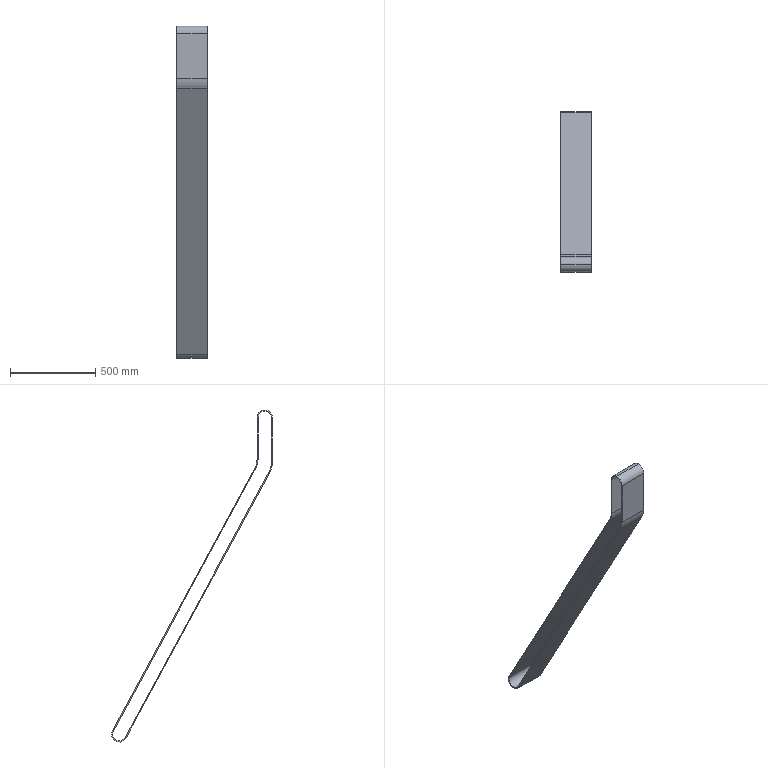Part | NX | 1 solid | 20 faces | box 180 x 945 x 1950 mm | volume 4768018 mm3 | cylinder 10 | plane 10 | commonest cylinder face diameters 78 x3 90 x3 240 x2 228 x1 252 x1
STEP:
#1=CARTESIAN_POINT('',(220.674,-610.499,2425.086));
#2=VERTEX_POINT('',#1);
#3=CARTESIAN_POINT('',(220.674,-649.499,2464.086));
#4=VERTEX_POINT('',#3);
#5=CARTESIAN_POINT('',(220.674,-649.499,2425.086));
#6=DIRECTION('',(1.,0.,0.));
#7=DIRECTION('',(0.,0.,-1.));
#8=AXIS2_PLACEMENT_3D('',#5,#6,#7);
#9=CIRCLE('',#8,39.);
#10=EDGE_CURVE('',#2,#4,#9,.T.);
#11=ORIENTED_EDGE('',*,*,#10,.T.);
#12=CARTESIAN_POINT('',(40.674,-649.499,2464.086));
#13=VERTEX_POINT('',#12);
#14=CARTESIAN_POINT('',(220.674,-649.499,2464.086));
#15=DIRECTION('',(-1.,0.,0.));
#16=VECTOR('',#15,1.);
#17=LINE('',#14,#16);
#18=EDGE_CURVE('',#4,#13,#17,.T.);
#19=ORIENTED_EDGE('',*,*,#18,.T.);
#20=CARTESIAN_POINT('',(40.674,-610.499,2425.086));
#21=VERTEX_POINT('',#20);
#22=CARTESIAN_POINT('',(40.674,-649.499,2425.086));
#23=DIRECTION('',(1.,0.,0.));
#24=DIRECTION('',(0.,0.,-1.));
#25=AXIS2_PLACEMENT_3D('',#22,#23,#24);
#26=CIRCLE('',#25,39.);
#27=EDGE_CURVE('',#21,#13,#26,.T.);
#28=ORIENTED_EDGE('',*,*,#27,.F.);
#29=CARTESIAN_POINT('',(220.674,-610.499,2425.086));
#30=DIRECTION('',(-1.,0.,0.));
#31=VECTOR('',#30,1.);
#32=LINE('',#29,#31);
#33=EDGE_CURVE('',#2,#21,#32,.T.);
#34=ORIENTED_EDGE('',*,*,#33,.F.);
#35=EDGE_LOOP('',(#11,#19,#28,#34));
#36=FACE_OUTER_BOUND('',#35,.T.);
#37=CARTESIAN_POINT('',(220.674,-649.499,2425.086));
#38=DIRECTION('',(-1.,0.,0.));
#39=DIRECTION('',(0.,0.,1.));
#40=AXIS2_PLACEMENT_3D('',#37,#38,#39);
#41=CYLINDRICAL_SURFACE('',#40,39.);
#42=ADVANCED_FACE('',(#36),#41,.F.);
#43=CARTESIAN_POINT('',(220.674,-649.499,2470.086));
#44=VERTEX_POINT('',#43);
#45=CARTESIAN_POINT('',(220.674,-694.499,2425.086));
#46=VERTEX_POINT('',#45);
#47=CARTESIAN_POINT('',(220.674,-649.499,2425.086));
#48=DIRECTION('',(1.,0.,0.));
#49=DIRECTION('',(0.,0.,-1.));
#50=AXIS2_PLACEMENT_3D('',#47,#48,#49);
#51=CIRCLE('',#50,45.);
#52=EDGE_CURVE('',#44,#46,#51,.T.);
#53=ORIENTED_EDGE('',*,*,#52,.F.);
#54=CARTESIAN_POINT('',(40.674,-649.499,2470.086));
#55=VERTEX_POINT('',#54);
#56=CARTESIAN_POINT('',(220.674,-649.499,2470.086));
#57=DIRECTION('',(-1.,0.,0.));
#58=VECTOR('',#57,1.);
#59=LINE('',#56,#58);
#60=EDGE_CURVE('',#44,#55,#59,.T.);
#61=ORIENTED_EDGE('',*,*,#60,.T.);
#62=CARTESIAN_POINT('',(40.674,-694.499,2425.086));
#63=VERTEX_POINT('',#62);
#64=CARTESIAN_POINT('',(40.674,-649.499,2425.086));
#65=DIRECTION('',(1.,0.,0.));
#66=DIRECTION('',(0.,0.,-1.));
#67=AXIS2_PLACEMENT_3D('',#64,#65,#66);
#68=CIRCLE('',#67,45.);
#69=EDGE_CURVE('',#55,#63,#68,.T.);
#70=ORIENTED_EDGE('',*,*,#69,.T.);
#71=CARTESIAN_POINT('',(220.674,-694.499,2425.086));
#72=DIRECTION('',(-1.,0.,0.));
#73=VECTOR('',#72,1.);
#74=LINE('',#71,#73);
#75=EDGE_CURVE('',#46,#63,#74,.T.);
#76=ORIENTED_EDGE('',*,*,#75,.F.);
#77=EDGE_LOOP('',(#53,#61,#70,#76));
#78=FACE_OUTER_BOUND('',#77,.T.);
#79=CARTESIAN_POINT('',(220.674,-649.499,2425.086));
#80=DIRECTION('',(-1.,0.,0.));
#81=DIRECTION('',(0.,0.,1.));
#82=AXIS2_PLACEMENT_3D('',#79,#80,#81);
#83=CYLINDRICAL_SURFACE('',#82,45.);
#84=ADVANCED_FACE('',(#78),#83,.T.);
#85=CARTESIAN_POINT('',(220.674,-590.01,2127.924));
#86=VERTEX_POINT('',#85);
#87=CARTESIAN_POINT('',(220.674,-604.499,2185.086));
#88=VERTEX_POINT('',#87);
#89=CARTESIAN_POINT('',(220.674,-484.499,2185.086));
#90=DIRECTION('',(-1.,0.,0.));
#91=DIRECTION('',(0.,0.,-1.));
#92=AXIS2_PLACEMENT_3D('',#89,#90,#91);
#93=CIRCLE('',#92,120.);
#94=EDGE_CURVE('',#86,#88,#93,.T.);
#95=ORIENTED_EDGE('',*,*,#94,.T.);
#96=CARTESIAN_POINT('',(220.674,-604.499,2425.086));
#97=VERTEX_POINT('',#96);
#98=CARTESIAN_POINT('',(220.674,-604.499,2425.086));
#99=DIRECTION('',(0.,0.,1.));
#100=VECTOR('',#99,1.);
#101=LINE('',#98,#100);
#102=EDGE_CURVE('',#88,#97,#101,.T.);
#103=ORIENTED_EDGE('',*,*,#102,.T.);
#104=CARTESIAN_POINT('',(220.674,-649.499,2425.086));
#105=DIRECTION('',(1.,0.,0.));
#106=DIRECTION('',(0.,0.,-1.));
#107=AXIS2_PLACEMENT_3D('',#104,#105,#106);
#108=CIRCLE('',#107,45.);
#109=EDGE_CURVE('',#97,#44,#108,.T.);
#110=ORIENTED_EDGE('',*,*,#109,.T.);
#111=ORIENTED_EDGE('',*,*,#52,.T.);
#112=CARTESIAN_POINT('',(220.674,-694.499,2162.273));
#113=VERTEX_POINT('',#112);
#114=CARTESIAN_POINT('',(220.674,-694.499,2162.273));
#115=DIRECTION('',(0.,0.,-1.));
#116=VECTOR('',#115,1.);
#117=LINE('',#114,#116);
#118=EDGE_CURVE('',#46,#113,#117,.T.);
#119=ORIENTED_EDGE('',*,*,#118,.T.);
#120=CARTESIAN_POINT('',(220.674,-680.01,2105.111));
#121=VERTEX_POINT('',#120);
#122=CARTESIAN_POINT('',(220.674,-574.499,2162.273));
#123=DIRECTION('',(1.,0.,0.));
#124=DIRECTION('',(0.,0.,1.));
#125=AXIS2_PLACEMENT_3D('',#122,#123,#124);
#126=CIRCLE('',#125,120.);
#127=EDGE_CURVE('',#113,#121,#126,.T.);
#128=ORIENTED_EDGE('',*,*,#127,.T.);
#129=CARTESIAN_POINT('',(220.674,165.934,543.65));
#130=VERTEX_POINT('',#129);
#131=CARTESIAN_POINT('',(220.674,165.934,543.65));
#132=DIRECTION('',(0.,0.4763,-0.8793));
#133=VECTOR('',#132,1.);
#134=LINE('',#131,#133);
#135=EDGE_CURVE('',#121,#130,#134,.T.);
#136=ORIENTED_EDGE('',*,*,#135,.T.);
#137=CARTESIAN_POINT('',(220.674,245.067,586.522));
#138=VERTEX_POINT('',#137);
#139=CARTESIAN_POINT('',(220.674,205.501,565.086));
#140=DIRECTION('',(1.,0.,0.));
#141=DIRECTION('',(0.,0.,1.));
#142=AXIS2_PLACEMENT_3D('',#139,#140,#141);
#143=CIRCLE('',#142,45.);
#144=EDGE_CURVE('',#130,#138,#143,.T.);
#145=ORIENTED_EDGE('',*,*,#144,.T.);
#146=CARTESIAN_POINT('',(220.674,-590.01,2127.924));
#147=DIRECTION('',(0.,-0.4763,0.8793));
#148=VECTOR('',#147,1.);
#149=LINE('',#146,#148);
#150=EDGE_CURVE('',#138,#86,#149,.T.);
#151=ORIENTED_EDGE('',*,*,#150,.T.);
#152=EDGE_LOOP('',(#95,#103,#110,#111,#119,#128,#136,#145,#151));
#153=FACE_BOUND('',#152,.T.);
#154=CARTESIAN_POINT('',(220.674,-595.286,2125.066));
#155=VERTEX_POINT('',#154);
#156=CARTESIAN_POINT('',(220.674,-610.499,2185.086));
#157=VERTEX_POINT('',#156);
#158=CARTESIAN_POINT('',(220.674,-484.499,2185.086));
#159=DIRECTION('',(-1.,0.,0.));
#160=DIRECTION('',(0.,0.,-1.));
#161=AXIS2_PLACEMENT_3D('',#158,#159,#160);
#162=CIRCLE('',#161,126.);
#163=EDGE_CURVE('',#155,#157,#162,.T.);
#164=ORIENTED_EDGE('',*,*,#163,.F.);
#165=CARTESIAN_POINT('',(220.674,239.792,583.664));
#166=VERTEX_POINT('',#165);
#167=CARTESIAN_POINT('',(220.674,-595.286,2125.066));
#168=DIRECTION('',(0.,-0.4763,0.8793));
#169=VECTOR('',#168,1.);
#170=LINE('',#167,#169);
#171=EDGE_CURVE('',#166,#155,#170,.T.);
#172=ORIENTED_EDGE('',*,*,#171,.F.);
#173=CARTESIAN_POINT('',(220.674,171.21,546.509));
#174=VERTEX_POINT('',#173);
#175=CARTESIAN_POINT('',(220.674,205.501,565.086));
#176=DIRECTION('',(1.,0.,0.));
#177=DIRECTION('',(0.,0.,-1.));
#178=AXIS2_PLACEMENT_3D('',#175,#176,#177);
#179=CIRCLE('',#178,39.);
#180=EDGE_CURVE('',#174,#166,#179,.T.);
#181=ORIENTED_EDGE('',*,*,#180,.F.);
#182=CARTESIAN_POINT('',(220.674,-674.734,2107.969));
#183=VERTEX_POINT('',#182);
#184=CARTESIAN_POINT('',(220.674,171.21,546.509));
#185=DIRECTION('',(0.,0.4763,-0.8793));
#186=VECTOR('',#185,1.);
#187=LINE('',#184,#186);
#188=EDGE_CURVE('',#183,#174,#187,.T.);
#189=ORIENTED_EDGE('',*,*,#188,.F.);
#190=CARTESIAN_POINT('',(220.674,-688.499,2162.273));
#191=VERTEX_POINT('',#190);
#192=CARTESIAN_POINT('',(220.674,-574.499,2162.273));
#193=DIRECTION('',(1.,0.,0.));
#194=DIRECTION('',(0.,0.,-1.));
#195=AXIS2_PLACEMENT_3D('',#192,#193,#194);
#196=CIRCLE('',#195,114.);
#197=EDGE_CURVE('',#191,#183,#196,.T.);
#198=ORIENTED_EDGE('',*,*,#197,.F.);
#199=CARTESIAN_POINT('',(220.674,-688.499,2425.086));
#200=VERTEX_POINT('',#199);
#201=CARTESIAN_POINT('',(220.674,-688.499,2162.273));
#202=DIRECTION('',(0.,0.,-1.));
#203=VECTOR('',#202,1.);
#204=LINE('',#201,#203);
#205=EDGE_CURVE('',#200,#191,#204,.T.);
#206=ORIENTED_EDGE('',*,*,#205,.F.);
#207=CARTESIAN_POINT('',(220.674,-649.499,2425.086));
#208=DIRECTION('',(1.,0.,0.));
#209=DIRECTION('',(0.,0.,-1.));
#210=AXIS2_PLACEMENT_3D('',#207,#208,#209);
#211=CIRCLE('',#210,39.);
#212=EDGE_CURVE('',#4,#200,#211,.T.);
#213=ORIENTED_EDGE('',*,*,#212,.F.);
#214=ORIENTED_EDGE('',*,*,#10,.F.);
#215=CARTESIAN_POINT('',(220.674,-610.499,2425.086));
#216=DIRECTION('',(0.,0.,1.));
#217=VECTOR('',#216,1.);
#218=LINE('',#215,#217);
#219=EDGE_CURVE('',#157,#2,#218,.T.);
#220=ORIENTED_EDGE('',*,*,#219,.F.);
#221=EDGE_LOOP('',(#164,#172,#181,#189,#198,#206,#213,#214,#220));
#222=FACE_BOUND('',#221,.T.);
#223=CARTESIAN_POINT('',(220.674,-484.499,2185.086));
#224=DIRECTION('',(-1.,0.,0.));
#225=DIRECTION('',(0.,0.,1.));
#226=AXIS2_PLACEMENT_3D('',#223,#224,#225);
#227=PLANE('',#226);
#228=ADVANCED_FACE('',(#153,#222),#227,.F.);
#229=CARTESIAN_POINT('',(40.674,-590.01,2127.924));
#230=VERTEX_POINT('',#229);
#231=CARTESIAN_POINT('',(40.674,-604.499,2185.086));
#232=VERTEX_POINT('',#231);
#233=CARTESIAN_POINT('',(40.674,-484.499,2185.086));
#234=DIRECTION('',(-1.,0.,0.));
#235=DIRECTION('',(0.,0.,-1.));
#236=AXIS2_PLACEMENT_3D('',#233,#234,#235);
#237=CIRCLE('',#236,120.);
#238=EDGE_CURVE('',#230,#232,#237,.T.);
#239=ORIENTED_EDGE('',*,*,#238,.F.);
#240=CARTESIAN_POINT('',(40.674,245.067,586.522));
#241=VERTEX_POINT('',#240);
#242=CARTESIAN_POINT('',(40.674,-590.01,2127.924));
#243=DIRECTION('',(0.,-0.4763,0.8793));
#244=VECTOR('',#243,1.);
#245=LINE('',#242,#244);
#246=EDGE_CURVE('',#241,#230,#245,.T.);
#247=ORIENTED_EDGE('',*,*,#246,.F.);
#248=CARTESIAN_POINT('',(40.674,165.934,543.65));
#249=VERTEX_POINT('',#248);
#250=CARTESIAN_POINT('',(40.674,205.501,565.086));
#251=DIRECTION('',(1.,0.,0.));
#252=DIRECTION('',(0.,0.,1.));
#253=AXIS2_PLACEMENT_3D('',#250,#251,#252);
#254=CIRCLE('',#253,45.);
#255=EDGE_CURVE('',#249,#241,#254,.T.);
#256=ORIENTED_EDGE('',*,*,#255,.F.);
#257=CARTESIAN_POINT('',(40.674,-680.01,2105.111));
#258=VERTEX_POINT('',#257);
#259=CARTESIAN_POINT('',(40.674,165.934,543.65));
#260=DIRECTION('',(0.,0.4763,-0.8793));
#261=VECTOR('',#260,1.);
#262=LINE('',#259,#261);
#263=EDGE_CURVE('',#258,#249,#262,.T.);
#264=ORIENTED_EDGE('',*,*,#263,.F.);
#265=CARTESIAN_POINT('',(40.674,-694.499,2162.273));
#266=VERTEX_POINT('',#265);
#267=CARTESIAN_POINT('',(40.674,-574.499,2162.273));
#268=DIRECTION('',(1.,0.,0.));
#269=DIRECTION('',(0.,0.,1.));
#270=AXIS2_PLACEMENT_3D('',#267,#268,#269);
#271=CIRCLE('',#270,120.);
#272=EDGE_CURVE('',#266,#258,#271,.T.);
#273=ORIENTED_EDGE('',*,*,#272,.F.);
#274=CARTESIAN_POINT('',(40.674,-694.499,2162.273));
#275=DIRECTION('',(0.,0.,-1.));
#276=VECTOR('',#275,1.);
#277=LINE('',#274,#276);
#278=EDGE_CURVE('',#63,#266,#277,.T.);
#279=ORIENTED_EDGE('',*,*,#278,.F.);
#280=ORIENTED_EDGE('',*,*,#69,.F.);
#281=CARTESIAN_POINT('',(40.674,-604.499,2425.086));
#282=VERTEX_POINT('',#281);
#283=CARTESIAN_POINT('',(40.674,-649.499,2425.086));
#284=DIRECTION('',(1.,0.,0.));
#285=DIRECTION('',(0.,0.,-1.));
#286=AXIS2_PLACEMENT_3D('',#283,#284,#285);
#287=CIRCLE('',#286,45.);
#288=EDGE_CURVE('',#282,#55,#287,.T.);
#289=ORIENTED_EDGE('',*,*,#288,.F.);
#290=CARTESIAN_POINT('',(40.674,-604.499,2425.086));
#291=DIRECTION('',(0.,0.,1.));
#292=VECTOR('',#291,1.);
#293=LINE('',#290,#292);
#294=EDGE_CURVE('',#232,#282,#293,.T.);
#295=ORIENTED_EDGE('',*,*,#294,.F.);
#296=EDGE_LOOP('',(#239,#247,#256,#264,#273,#279,#280,#289,#295));
#297=FACE_BOUND('',#296,.T.);
#298=CARTESIAN_POINT('',(40.674,239.792,583.664));
#299=VERTEX_POINT('',#298);
#300=CARTESIAN_POINT('',(40.674,-595.286,2125.066));
#301=VERTEX_POINT('',#300);
#302=CARTESIAN_POINT('',(40.674,-595.286,2125.066));
#303=DIRECTION('',(0.,-0.4763,0.8793));
#304=VECTOR('',#303,1.);
#305=LINE('',#302,#304);
#306=EDGE_CURVE('',#299,#301,#305,.T.);
#307=ORIENTED_EDGE('',*,*,#306,.T.);
#308=CARTESIAN_POINT('',(40.674,-610.499,2185.086));
#309=VERTEX_POINT('',#308);
#310=CARTESIAN_POINT('',(40.674,-484.499,2185.086));
#311=DIRECTION('',(-1.,0.,0.));
#312=DIRECTION('',(0.,0.,-1.));
#313=AXIS2_PLACEMENT_3D('',#310,#311,#312);
#314=CIRCLE('',#313,126.);
#315=EDGE_CURVE('',#301,#309,#314,.T.);
#316=ORIENTED_EDGE('',*,*,#315,.T.);
#317=CARTESIAN_POINT('',(40.674,-610.499,2425.086));
#318=DIRECTION('',(0.,0.,1.));
#319=VECTOR('',#318,1.);
#320=LINE('',#317,#319);
#321=EDGE_CURVE('',#309,#21,#320,.T.);
#322=ORIENTED_EDGE('',*,*,#321,.T.);
#323=ORIENTED_EDGE('',*,*,#27,.T.);
#324=CARTESIAN_POINT('',(40.674,-688.499,2425.086));
#325=VERTEX_POINT('',#324);
#326=CARTESIAN_POINT('',(40.674,-649.499,2425.086));
#327=DIRECTION('',(1.,0.,0.));
#328=DIRECTION('',(0.,0.,-1.));
#329=AXIS2_PLACEMENT_3D('',#326,#327,#328);
#330=CIRCLE('',#329,39.);
#331=EDGE_CURVE('',#13,#325,#330,.T.);
#332=ORIENTED_EDGE('',*,*,#331,.T.);
#333=CARTESIAN_POINT('',(40.674,-688.499,2162.273));
#334=VERTEX_POINT('',#333);
#335=CARTESIAN_POINT('',(40.674,-688.499,2162.273));
#336=DIRECTION('',(0.,0.,-1.));
#337=VECTOR('',#336,1.);
#338=LINE('',#335,#337);
#339=EDGE_CURVE('',#325,#334,#338,.T.);
#340=ORIENTED_EDGE('',*,*,#339,.T.);
#341=CARTESIAN_POINT('',(40.674,-674.734,2107.969));
#342=VERTEX_POINT('',#341);
#343=CARTESIAN_POINT('',(40.674,-574.499,2162.273));
#344=DIRECTION('',(1.,0.,0.));
#345=DIRECTION('',(0.,0.,-1.));
#346=AXIS2_PLACEMENT_3D('',#343,#344,#345);
#347=CIRCLE('',#346,114.);
#348=EDGE_CURVE('',#334,#342,#347,.T.);
#349=ORIENTED_EDGE('',*,*,#348,.T.);
#350=CARTESIAN_POINT('',(40.674,171.21,546.509));
#351=VERTEX_POINT('',#350);
#352=CARTESIAN_POINT('',(40.674,171.21,546.509));
#353=DIRECTION('',(0.,0.4763,-0.8793));
#354=VECTOR('',#353,1.);
#355=LINE('',#352,#354);
#356=EDGE_CURVE('',#342,#351,#355,.T.);
#357=ORIENTED_EDGE('',*,*,#356,.T.);
#358=CARTESIAN_POINT('',(40.674,205.501,565.086));
#359=DIRECTION('',(1.,0.,0.));
#360=DIRECTION('',(0.,0.,-1.));
#361=AXIS2_PLACEMENT_3D('',#358,#359,#360);
#362=CIRCLE('',#361,39.);
#363=EDGE_CURVE('',#351,#299,#362,.T.);
#364=ORIENTED_EDGE('',*,*,#363,.T.);
#365=EDGE_LOOP('',(#307,#316,#322,#323,#332,#340,#349,#357,#364));
#366=FACE_BOUND('',#365,.T.);
#367=CARTESIAN_POINT('',(40.674,-484.499,2185.086));
#368=DIRECTION('',(-1.,0.,0.));
#369=DIRECTION('',(0.,0.,1.));
#370=AXIS2_PLACEMENT_3D('',#367,#368,#369);
#371=PLANE('',#370);
#372=ADVANCED_FACE('',(#297,#366),#371,.T.);
#373=ORIENTED_EDGE('',*,*,#238,.T.);
#374=CARTESIAN_POINT('',(220.674,-604.499,2185.086));
#375=DIRECTION('',(-1.,0.,0.));
#376=VECTOR('',#375,1.);
#377=LINE('',#374,#376);
#378=EDGE_CURVE('',#88,#232,#377,.T.);
#379=ORIENTED_EDGE('',*,*,#378,.F.);
#380=ORIENTED_EDGE('',*,*,#94,.F.);
#381=CARTESIAN_POINT('',(220.674,-590.01,2127.924));
#382=DIRECTION('',(-1.,0.,0.));
#383=VECTOR('',#382,1.);
#384=LINE('',#381,#383);
#385=EDGE_CURVE('',#86,#230,#384,.T.);
#386=ORIENTED_EDGE('',*,*,#385,.T.);
#387=EDGE_LOOP('',(#373,#379,#380,#386));
#388=FACE_OUTER_BOUND('',#387,.T.);
#389=CARTESIAN_POINT('',(220.674,-484.499,2185.086));
#390=DIRECTION('',(-1.,0.,0.));
#391=DIRECTION('',(0.,0.,1.));
#392=AXIS2_PLACEMENT_3D('',#389,#390,#391);
#393=CYLINDRICAL_SURFACE('',#392,120.);
#394=ADVANCED_FACE('',(#388),#393,.F.);
#395=ORIENTED_EDGE('',*,*,#294,.T.);
#396=CARTESIAN_POINT('',(220.674,-604.499,2425.086));
#397=DIRECTION('',(-1.,0.,0.));
#398=VECTOR('',#397,1.);
#399=LINE('',#396,#398);
#400=EDGE_CURVE('',#97,#282,#399,.T.);
#401=ORIENTED_EDGE('',*,*,#400,.F.);
#402=ORIENTED_EDGE('',*,*,#102,.F.);
#403=ORIENTED_EDGE('',*,*,#378,.T.);
#404=EDGE_LOOP('',(#395,#401,#402,#403));
#405=FACE_OUTER_BOUND('',#404,.T.);
#406=CARTESIAN_POINT('',(220.674,-604.499,2425.086));
#407=DIRECTION('',(0.,-1.,0.));
#408=DIRECTION('',(0.,0.,-1.));
#409=AXIS2_PLACEMENT_3D('',#406,#407,#408);
#410=PLANE('',#409);
#411=ADVANCED_FACE('',(#405),#410,.F.);
#412=ORIENTED_EDGE('',*,*,#60,.F.);
#413=ORIENTED_EDGE('',*,*,#109,.F.);
#414=ORIENTED_EDGE('',*,*,#400,.T.);
#415=ORIENTED_EDGE('',*,*,#288,.T.);
#416=EDGE_LOOP('',(#412,#413,#414,#415));
#417=FACE_OUTER_BOUND('',#416,.T.);
#418=CARTESIAN_POINT('',(220.674,-649.499,2425.086));
#419=DIRECTION('',(-1.,0.,0.));
#420=DIRECTION('',(0.,0.,1.));
#421=AXIS2_PLACEMENT_3D('',#418,#419,#420);
#422=CYLINDRICAL_SURFACE('',#421,45.);
#423=ADVANCED_FACE('',(#417),#422,.T.);
#424=ORIENTED_EDGE('',*,*,#278,.T.);
#425=CARTESIAN_POINT('',(220.674,-694.499,2162.273));
#426=DIRECTION('',(-1.,0.,0.));
#427=VECTOR('',#426,1.);
#428=LINE('',#425,#427);
#429=EDGE_CURVE('',#113,#266,#428,.T.);
#430=ORIENTED_EDGE('',*,*,#429,.F.);
#431=ORIENTED_EDGE('',*,*,#118,.F.);
#432=ORIENTED_EDGE('',*,*,#75,.T.);
#433=EDGE_LOOP('',(#424,#430,#431,#432));
#434=FACE_OUTER_BOUND('',#433,.T.);
#435=CARTESIAN_POINT('',(220.674,-694.499,2162.273));
#436=DIRECTION('',(0.,1.,0.));
#437=DIRECTION('',(0.,0.,1.));
#438=AXIS2_PLACEMENT_3D('',#435,#436,#437);
#439=PLANE('',#438);
#440=ADVANCED_FACE('',(#434),#439,.F.);
#441=ORIENTED_EDGE('',*,*,#272,.T.);
#442=CARTESIAN_POINT('',(220.674,-680.01,2105.111));
#443=DIRECTION('',(-1.,0.,0.));
#444=VECTOR('',#443,1.);
#445=LINE('',#442,#444);
#446=EDGE_CURVE('',#121,#258,#445,.T.);
#447=ORIENTED_EDGE('',*,*,#446,.F.);
#448=ORIENTED_EDGE('',*,*,#127,.F.);
#449=ORIENTED_EDGE('',*,*,#429,.T.);
#450=EDGE_LOOP('',(#441,#447,#448,#449));
#451=FACE_OUTER_BOUND('',#450,.T.);
#452=CARTESIAN_POINT('',(220.674,-574.499,2162.273));
#453=DIRECTION('',(-1.,0.,0.));
#454=DIRECTION('',(0.,0.,1.));
#455=AXIS2_PLACEMENT_3D('',#452,#453,#454);
#456=CYLINDRICAL_SURFACE('',#455,120.);
#457=ADVANCED_FACE('',(#451),#456,.T.);
#458=ORIENTED_EDGE('',*,*,#263,.T.);
#459=CARTESIAN_POINT('',(220.674,165.934,543.65));
#460=DIRECTION('',(-1.,0.,0.));
#461=VECTOR('',#460,1.);
#462=LINE('',#459,#461);
#463=EDGE_CURVE('',#130,#249,#462,.T.);
#464=ORIENTED_EDGE('',*,*,#463,.F.);
#465=ORIENTED_EDGE('',*,*,#135,.F.);
#466=ORIENTED_EDGE('',*,*,#446,.T.);
#467=EDGE_LOOP('',(#458,#464,#465,#466));
#468=FACE_OUTER_BOUND('',#467,.T.);
#469=CARTESIAN_POINT('',(220.674,165.934,543.65));
#470=DIRECTION('',(0.,0.8793,0.4763));
#471=DIRECTION('',(0.,-0.4763,0.8793));
#472=AXIS2_PLACEMENT_3D('',#469,#470,#471);
#473=PLANE('',#472);
#474=ADVANCED_FACE('',(#468),#473,.F.);
#475=ORIENTED_EDGE('',*,*,#255,.T.);
#476=CARTESIAN_POINT('',(220.674,245.067,586.522));
#477=DIRECTION('',(-1.,0.,0.));
#478=VECTOR('',#477,1.);
#479=LINE('',#476,#478);
#480=EDGE_CURVE('',#138,#241,#479,.T.);
#481=ORIENTED_EDGE('',*,*,#480,.F.);
#482=ORIENTED_EDGE('',*,*,#144,.F.);
#483=ORIENTED_EDGE('',*,*,#463,.T.);
#484=EDGE_LOOP('',(#475,#481,#482,#483));
#485=FACE_OUTER_BOUND('',#484,.T.);
#486=CARTESIAN_POINT('',(220.674,205.501,565.086));
#487=DIRECTION('',(-1.,0.,0.));
#488=DIRECTION('',(0.,0.,1.));
#489=AXIS2_PLACEMENT_3D('',#486,#487,#488);
#490=CYLINDRICAL_SURFACE('',#489,45.);
#491=ADVANCED_FACE('',(#485),#490,.T.);
#492=ORIENTED_EDGE('',*,*,#246,.T.);
#493=ORIENTED_EDGE('',*,*,#385,.F.);
#494=ORIENTED_EDGE('',*,*,#150,.F.);
#495=ORIENTED_EDGE('',*,*,#480,.T.);
#496=EDGE_LOOP('',(#492,#493,#494,#495));
#497=FACE_OUTER_BOUND('',#496,.T.);
#498=CARTESIAN_POINT('',(220.674,-590.01,2127.924));
#499=DIRECTION('',(0.,-0.8793,-0.4763));
#500=DIRECTION('',(0.,0.4763,-0.8793));
#501=AXIS2_PLACEMENT_3D('',#498,#499,#500);
#502=PLANE('',#501);
#503=ADVANCED_FACE('',(#497),#502,.F.);
#504=ORIENTED_EDGE('',*,*,#315,.F.);
#505=CARTESIAN_POINT('',(220.674,-595.286,2125.066));
#506=DIRECTION('',(-1.,0.,0.));
#507=VECTOR('',#506,1.);
#508=LINE('',#505,#507);
#509=EDGE_CURVE('',#155,#301,#508,.T.);
#510=ORIENTED_EDGE('',*,*,#509,.F.);
#511=ORIENTED_EDGE('',*,*,#163,.T.);
#512=CARTESIAN_POINT('',(220.674,-610.499,2185.086));
#513=DIRECTION('',(-1.,0.,0.));
#514=VECTOR('',#513,1.);
#515=LINE('',#512,#514);
#516=EDGE_CURVE('',#157,#309,#515,.T.);
#517=ORIENTED_EDGE('',*,*,#516,.T.);
#518=EDGE_LOOP('',(#504,#510,#511,#517));
#519=FACE_OUTER_BOUND('',#518,.T.);
#520=CARTESIAN_POINT('',(220.674,-484.499,2185.086));
#521=DIRECTION('',(-1.,0.,0.));
#522=DIRECTION('',(0.,0.,1.));
#523=AXIS2_PLACEMENT_3D('',#520,#521,#522);
#524=CYLINDRICAL_SURFACE('',#523,126.);
#525=ADVANCED_FACE('',(#519),#524,.T.);
#526=ORIENTED_EDGE('',*,*,#321,.F.);
#527=ORIENTED_EDGE('',*,*,#516,.F.);
#528=ORIENTED_EDGE('',*,*,#219,.T.);
#529=ORIENTED_EDGE('',*,*,#33,.T.);
#530=EDGE_LOOP('',(#526,#527,#528,#529));
#531=FACE_OUTER_BOUND('',#530,.T.);
#532=CARTESIAN_POINT('',(220.674,-610.499,2425.086));
#533=DIRECTION('',(0.,-1.,0.));
#534=DIRECTION('',(0.,0.,-1.));
#535=AXIS2_PLACEMENT_3D('',#532,#533,#534);
#536=PLANE('',#535);
#537=ADVANCED_FACE('',(#531),#536,.T.);
#538=ORIENTED_EDGE('',*,*,#18,.F.);
#539=ORIENTED_EDGE('',*,*,#212,.T.);
#540=CARTESIAN_POINT('',(220.674,-688.499,2425.086));
#541=DIRECTION('',(-1.,0.,0.));
#542=VECTOR('',#541,1.);
#543=LINE('',#540,#542);
#544=EDGE_CURVE('',#200,#325,#543,.T.);
#545=ORIENTED_EDGE('',*,*,#544,.T.);
#546=ORIENTED_EDGE('',*,*,#331,.F.);
#547=EDGE_LOOP('',(#538,#539,#545,#546));
#548=FACE_OUTER_BOUND('',#547,.T.);
#549=CARTESIAN_POINT('',(220.674,-649.499,2425.086));
#550=DIRECTION('',(-1.,0.,0.));
#551=DIRECTION('',(0.,0.,1.));
#552=AXIS2_PLACEMENT_3D('',#549,#550,#551);
#553=CYLINDRICAL_SURFACE('',#552,39.);
#554=ADVANCED_FACE('',(#548),#553,.F.);
#555=ORIENTED_EDGE('',*,*,#339,.F.);
#556=ORIENTED_EDGE('',*,*,#544,.F.);
#557=ORIENTED_EDGE('',*,*,#205,.T.);
#558=CARTESIAN_POINT('',(220.674,-688.499,2162.273));
#559=DIRECTION('',(-1.,0.,0.));
#560=VECTOR('',#559,1.);
#561=LINE('',#558,#560);
#562=EDGE_CURVE('',#191,#334,#561,.T.);
#563=ORIENTED_EDGE('',*,*,#562,.T.);
#564=EDGE_LOOP('',(#555,#556,#557,#563));
#565=FACE_OUTER_BOUND('',#564,.T.);
#566=CARTESIAN_POINT('',(220.674,-688.499,2162.273));
#567=DIRECTION('',(0.,1.,0.));
#568=DIRECTION('',(0.,0.,1.));
#569=AXIS2_PLACEMENT_3D('',#566,#567,#568);
#570=PLANE('',#569);
#571=ADVANCED_FACE('',(#565),#570,.T.);
#572=ORIENTED_EDGE('',*,*,#348,.F.);
#573=ORIENTED_EDGE('',*,*,#562,.F.);
#574=ORIENTED_EDGE('',*,*,#197,.T.);
#575=CARTESIAN_POINT('',(220.674,-674.734,2107.969));
#576=DIRECTION('',(-1.,0.,0.));
#577=VECTOR('',#576,1.);
#578=LINE('',#575,#577);
#579=EDGE_CURVE('',#183,#342,#578,.T.);
#580=ORIENTED_EDGE('',*,*,#579,.T.);
#581=EDGE_LOOP('',(#572,#573,#574,#580));
#582=FACE_OUTER_BOUND('',#581,.T.);
#583=CARTESIAN_POINT('',(220.674,-574.499,2162.273));
#584=DIRECTION('',(-1.,0.,0.));
#585=DIRECTION('',(0.,0.,1.));
#586=AXIS2_PLACEMENT_3D('',#583,#584,#585);
#587=CYLINDRICAL_SURFACE('',#586,114.);
#588=ADVANCED_FACE('',(#582),#587,.F.);
#589=ORIENTED_EDGE('',*,*,#356,.F.);
#590=ORIENTED_EDGE('',*,*,#579,.F.);
#591=ORIENTED_EDGE('',*,*,#188,.T.);
#592=CARTESIAN_POINT('',(220.674,171.21,546.509));
#593=DIRECTION('',(-1.,0.,0.));
#594=VECTOR('',#593,1.);
#595=LINE('',#592,#594);
#596=EDGE_CURVE('',#174,#351,#595,.T.);
#597=ORIENTED_EDGE('',*,*,#596,.T.);
#598=EDGE_LOOP('',(#589,#590,#591,#597));
#599=FACE_OUTER_BOUND('',#598,.T.);
#600=CARTESIAN_POINT('',(220.674,171.21,546.509));
#601=DIRECTION('',(0.,0.8793,0.4763));
#602=DIRECTION('',(0.,-0.4763,0.8793));
#603=AXIS2_PLACEMENT_3D('',#600,#601,#602);
#604=PLANE('',#603);
#605=ADVANCED_FACE('',(#599),#604,.T.);
#606=ORIENTED_EDGE('',*,*,#363,.F.);
#607=ORIENTED_EDGE('',*,*,#596,.F.);
#608=ORIENTED_EDGE('',*,*,#180,.T.);
#609=CARTESIAN_POINT('',(220.674,239.792,583.664));
#610=DIRECTION('',(-1.,0.,0.));
#611=VECTOR('',#610,1.);
#612=LINE('',#609,#611);
#613=EDGE_CURVE('',#166,#299,#612,.T.);
#614=ORIENTED_EDGE('',*,*,#613,.T.);
#615=EDGE_LOOP('',(#606,#607,#608,#614));
#616=FACE_OUTER_BOUND('',#615,.T.);
#617=CARTESIAN_POINT('',(220.674,205.501,565.086));
#618=DIRECTION('',(-1.,0.,0.));
#619=DIRECTION('',(0.,0.,1.));
#620=AXIS2_PLACEMENT_3D('',#617,#618,#619);
#621=CYLINDRICAL_SURFACE('',#620,39.);
#622=ADVANCED_FACE('',(#616),#621,.F.);
#623=ORIENTED_EDGE('',*,*,#306,.F.);
#624=ORIENTED_EDGE('',*,*,#613,.F.);
#625=ORIENTED_EDGE('',*,*,#171,.T.);
#626=ORIENTED_EDGE('',*,*,#509,.T.);
#627=EDGE_LOOP('',(#623,#624,#625,#626));
#628=FACE_OUTER_BOUND('',#627,.T.);
#629=CARTESIAN_POINT('',(220.674,-595.286,2125.066));
#630=DIRECTION('',(0.,-0.8793,-0.4763));
#631=DIRECTION('',(0.,0.4763,-0.8793));
#632=AXIS2_PLACEMENT_3D('',#629,#630,#631);
#633=PLANE('',#632);
#634=ADVANCED_FACE('',(#628),#633,.T.);
#635=CLOSED_SHELL('',(#42,#84,#228,#372,#394,#411,#423,#440,#457,#474,#491,#503,#525,#537,#554,#571,#588,#605,#622,#634));
#636=MANIFOLD_SOLID_BREP('',#635);
#637=(LENGTH_UNIT()NAMED_UNIT(*)SI_UNIT(.MILLI.,.METRE.));
#638=UNCERTAINTY_MEASURE_WITH_UNIT(LENGTH_MEASURE(0.00002),#637,'','');
#639=(NAMED_UNIT(*)PLANE_ANGLE_UNIT()SI_UNIT($,.RADIAN.));
#640=PLANE_ANGLE_MEASURE_WITH_UNIT(PLANE_ANGLE_MEASURE(0.01745),#639);
#641=DIMENSIONAL_EXPONENTS(0.,0.,0.,0.,0.,0.,0.);
#642=(CONVERSION_BASED_UNIT('DEGREE',#640)NAMED_UNIT(#641)PLANE_ANGLE_UNIT());
#643=(NAMED_UNIT(*)SI_UNIT($,.STERADIAN.)SOLID_ANGLE_UNIT());
#644=(GEOMETRIC_REPRESENTATION_CONTEXT(3)GLOBAL_UNCERTAINTY_ASSIGNED_CONTEXT((#638))GLOBAL_UNIT_ASSIGNED_CONTEXT((#637,#642,#643))REPRESENTATION_CONTEXT('',''));
#645=ADVANCED_BREP_SHAPE_REPRESENTATION('',(#636),#644);